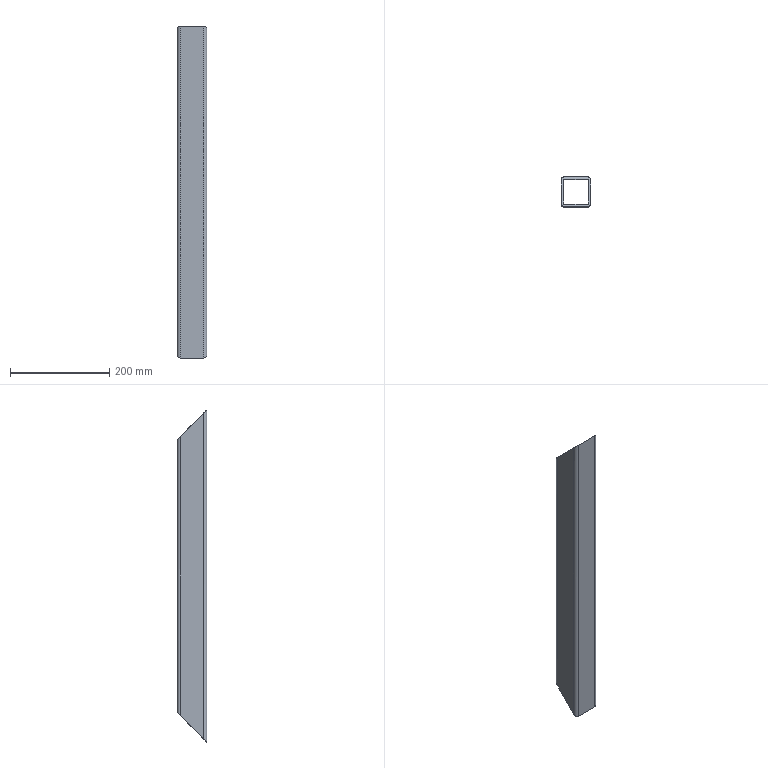Part | STEP file | Positioning_id1438_x_t | 1 solid | 14 faces | box 60 x 60 x 670 mm | volume 652149 mm3 | plane 10 | cylinder 4 | commonest cylinder face diameters 12 x4
STEP:
#1=CARTESIAN_POINT('',(0.,0.,0.));
#2=DIRECTION('',(0.,0.,1.));
#3=DIRECTION('',(1.,0.,0.));
#4=AXIS2_PLACEMENT_3D('',#1,#2,#3);
#5=CARTESIAN_POINT('',(-1086.002,-745.,-132.534));
#6=VERTEX_POINT('',#5);
#7=CARTESIAN_POINT('',(-1086.002,-695.,-82.534));
#8=VERTEX_POINT('',#7);
#9=CARTESIAN_POINT('',(-1086.002,-745.,-132.534));
#10=DIRECTION('',(0.,0.7071,0.7071));
#11=VECTOR('',#10,1.);
#12=LINE('',#9,#11);
#13=CARTESIAN_POINT('',(-1021.002,-750.,-137.534));
#14=DIRECTION('',(0.,-0.7071,0.7071));
#15=DIRECTION('',(0.,0.7071,0.7071));
#16=AXIS2_PLACEMENT_3D('',#13,#14,#15);
#17=PLANE('',#16);
#18=CARTESIAN_POINT('',(7.071,65.));
#19=DIRECTION('',(1.,0.));
#20=VECTOR('',#19,1.);
#21=LINE('',#18,#20);
#22=(GEOMETRIC_REPRESENTATION_CONTEXT(2)PARAMETRIC_REPRESENTATION_CONTEXT()REPRESENTATION_CONTEXT('',''));
#23=DEFINITIONAL_REPRESENTATION('',(#21),#22);
#24=PCURVE('',#17,#23);
#25=CARTESIAN_POINT('',(-1086.002,-745.,257.466));
#26=DIRECTION('',(-1.,0.,0.));
#27=DIRECTION('',(0.,1.,0.));
#28=AXIS2_PLACEMENT_3D('',#25,#26,#27);
#29=PLANE('',#28);
#30=CARTESIAN_POINT('',(0.,390.));
#31=DIRECTION('',(0.7071,-0.7071));
#32=VECTOR('',#31,1.);
#33=LINE('',#30,#32);
#34=(GEOMETRIC_REPRESENTATION_CONTEXT(2)PARAMETRIC_REPRESENTATION_CONTEXT()REPRESENTATION_CONTEXT('',''));
#35=DEFINITIONAL_REPRESENTATION('',(#33),#34);
#36=PCURVE('',#29,#35);
#37=SURFACE_CURVE('',#12,(#24,#36),.PCURVE_S1.);
#38=EDGE_CURVE('',#6,#8,#37,.T.);
#39=ORIENTED_EDGE('',*,*,#38,.F.);
#40=CARTESIAN_POINT('',(-1036.002,-745.,-132.534));
#41=VERTEX_POINT('',#40);
#42=CARTESIAN_POINT('',(-1036.002,-745.,-132.534));
#43=DIRECTION('',(-1.,0.,0.));
#44=VECTOR('',#43,1.);
#45=LINE('',#42,#44);
#46=CARTESIAN_POINT('',(7.071,15.));
#47=DIRECTION('',(0.,1.));
#48=VECTOR('',#47,1.);
#49=LINE('',#46,#48);
#50=(GEOMETRIC_REPRESENTATION_CONTEXT(2)PARAMETRIC_REPRESENTATION_CONTEXT()REPRESENTATION_CONTEXT('',''));
#51=DEFINITIONAL_REPRESENTATION('',(#49),#50);
#52=PCURVE('',#17,#51);
#53=CARTESIAN_POINT('',(-1061.002,-745.,257.466));
#54=DIRECTION('',(0.,-1.,0.));
#55=DIRECTION('',(-1.,0.,0.));
#56=AXIS2_PLACEMENT_3D('',#53,#54,#55);
#57=PLANE('',#56);
#58=CARTESIAN_POINT('',(-25.,390.));
#59=DIRECTION('',(1.,0.));
#60=VECTOR('',#59,1.);
#61=LINE('',#58,#60);
#62=(GEOMETRIC_REPRESENTATION_CONTEXT(2)PARAMETRIC_REPRESENTATION_CONTEXT()REPRESENTATION_CONTEXT('',''));
#63=DEFINITIONAL_REPRESENTATION('',(#61),#62);
#64=PCURVE('',#57,#63);
#65=SURFACE_CURVE('',#45,(#52,#64),.PCURVE_S1.);
#66=EDGE_CURVE('',#41,#6,#65,.T.);
#67=ORIENTED_EDGE('',*,*,#66,.F.);
#68=CARTESIAN_POINT('',(-1036.002,-695.,-82.534));
#69=VERTEX_POINT('',#68);
#70=CARTESIAN_POINT('',(-1036.002,-695.,-82.534));
#71=DIRECTION('',(0.,-0.7071,-0.7071));
#72=VECTOR('',#71,1.);
#73=LINE('',#70,#72);
#74=CARTESIAN_POINT('',(77.782,15.));
#75=DIRECTION('',(-1.,0.));
#76=VECTOR('',#75,1.);
#77=LINE('',#74,#76);
#78=(GEOMETRIC_REPRESENTATION_CONTEXT(2)PARAMETRIC_REPRESENTATION_CONTEXT()REPRESENTATION_CONTEXT('',''));
#79=DEFINITIONAL_REPRESENTATION('',(#77),#78);
#80=PCURVE('',#17,#79);
#81=CARTESIAN_POINT('',(-1036.002,-745.,257.466));
#82=DIRECTION('',(1.,0.,0.));
#83=DIRECTION('',(0.,-1.,0.));
#84=AXIS2_PLACEMENT_3D('',#81,#82,#83);
#85=PLANE('',#84);
#86=CARTESIAN_POINT('',(-50.,340.));
#87=DIRECTION('',(0.7071,0.7071));
#88=VECTOR('',#87,1.);
#89=LINE('',#86,#88);
#90=(GEOMETRIC_REPRESENTATION_CONTEXT(2)PARAMETRIC_REPRESENTATION_CONTEXT()REPRESENTATION_CONTEXT('',''));
#91=DEFINITIONAL_REPRESENTATION('',(#89),#90);
#92=PCURVE('',#85,#91);
#93=SURFACE_CURVE('',#73,(#80,#92),.PCURVE_S1.);
#94=EDGE_CURVE('',#69,#41,#93,.T.);
#95=ORIENTED_EDGE('',*,*,#94,.F.);
#96=CARTESIAN_POINT('',(-1086.002,-695.,-82.534));
#97=DIRECTION('',(1.,0.,0.));
#98=VECTOR('',#97,1.);
#99=LINE('',#96,#98);
#100=CARTESIAN_POINT('',(77.782,65.));
#101=DIRECTION('',(0.,-1.));
#102=VECTOR('',#101,1.);
#103=LINE('',#100,#102);
#104=(GEOMETRIC_REPRESENTATION_CONTEXT(2)PARAMETRIC_REPRESENTATION_CONTEXT()REPRESENTATION_CONTEXT('',''));
#105=DEFINITIONAL_REPRESENTATION('',(#103),#104);
#106=PCURVE('',#17,#105);
#107=CARTESIAN_POINT('',(-1061.002,-695.,257.466));
#108=DIRECTION('',(0.,1.,0.));
#109=DIRECTION('',(1.,0.,0.));
#110=AXIS2_PLACEMENT_3D('',#107,#108,#109);
#111=PLANE('',#110);
#112=CARTESIAN_POINT('',(-25.,340.));
#113=DIRECTION('',(1.,0.));
#114=VECTOR('',#113,1.);
#115=LINE('',#112,#114);
#116=(GEOMETRIC_REPRESENTATION_CONTEXT(2)PARAMETRIC_REPRESENTATION_CONTEXT()REPRESENTATION_CONTEXT('',''));
#117=DEFINITIONAL_REPRESENTATION('',(#115),#116);
#118=PCURVE('',#111,#117);
#119=SURFACE_CURVE('',#99,(#106,#118),.PCURVE_S1.);
#120=EDGE_CURVE('',#8,#69,#119,.T.);
#121=ORIENTED_EDGE('',*,*,#120,.F.);
#122=EDGE_LOOP('',(#39,#67,#95,#121));
#123=FACE_BOUND('',#122,.T.);
#124=CARTESIAN_POINT('',(-1085.002,-690.,-77.534));
#125=VERTEX_POINT('',#124);
#126=CARTESIAN_POINT('',(-1037.002,-690.,-77.534));
#127=VERTEX_POINT('',#126);
#128=CARTESIAN_POINT('',(-1085.002,-690.,-77.534));
#129=DIRECTION('',(1.,0.,0.));
#130=VECTOR('',#129,1.);
#131=LINE('',#128,#130);
#132=CARTESIAN_POINT('',(84.853,64.));
#133=DIRECTION('',(0.,-1.));
#134=VECTOR('',#133,1.);
#135=LINE('',#132,#134);
#136=(GEOMETRIC_REPRESENTATION_CONTEXT(2)PARAMETRIC_REPRESENTATION_CONTEXT()REPRESENTATION_CONTEXT('',''));
#137=DEFINITIONAL_REPRESENTATION('',(#135),#136);
#138=PCURVE('',#17,#137);
#139=CARTESIAN_POINT('',(-1061.002,-690.,257.466));
#140=DIRECTION('',(0.,1.,0.));
#141=DIRECTION('',(1.,0.,0.));
#142=AXIS2_PLACEMENT_3D('',#139,#140,#141);
#143=PLANE('',#142);
#144=CARTESIAN_POINT('',(-24.,335.));
#145=DIRECTION('',(1.,0.));
#146=VECTOR('',#145,1.);
#147=LINE('',#144,#146);
#148=(GEOMETRIC_REPRESENTATION_CONTEXT(2)PARAMETRIC_REPRESENTATION_CONTEXT()REPRESENTATION_CONTEXT('',''));
#149=DEFINITIONAL_REPRESENTATION('',(#147),#148);
#150=PCURVE('',#143,#149);
#151=SURFACE_CURVE('',#131,(#138,#150),.PCURVE_S1.);
#152=EDGE_CURVE('',#125,#127,#151,.T.);
#153=ORIENTED_EDGE('',*,*,#152,.T.);
#154=CARTESIAN_POINT('',(-1031.002,-696.,-83.534));
#155=VERTEX_POINT('',#154);
#156=CARTESIAN_POINT('',(-1037.002,-696.,-83.534));
#157=DIRECTION('',(0.,0.7071,-0.7071));
#158=DIRECTION('',(0.,-0.7071,-0.7071));
#159=AXIS2_PLACEMENT_3D('',#156,#157,#158);
#160=ELLIPSE('',#159,8.485,6.);
#161=CARTESIAN_POINT('',(67.882,16.));
#162=CARTESIAN_POINT('',(67.882,26.392));
#163=CARTESIAN_POINT('',(80.61,21.196));
#164=CARTESIAN_POINT('',(93.338,16.));
#165=CARTESIAN_POINT('',(80.61,10.804));
#166=CARTESIAN_POINT('',(67.882,5.608));
#167=CARTESIAN_POINT('',(67.882,16.));
#168=(BOUNDED_CURVE()B_SPLINE_CURVE(2,(#161,#162,#163,#164,#165,#166,#167),.UNSPECIFIED.,.T.,.F.)B_SPLINE_CURVE_WITH_KNOTS((1,2,2,2,2,1),(-2.094,0.,2.094,4.189,6.283,8.378),.UNSPECIFIED.)CURVE()GEOMETRIC_REPRESENTATION_ITEM()RATIONAL_B_SPLINE_CURVE((1.,0.5,1.,0.5,1.,0.5,1.))REPRESENTATION_ITEM(''));
#169=(GEOMETRIC_REPRESENTATION_CONTEXT(2)PARAMETRIC_REPRESENTATION_CONTEXT()REPRESENTATION_CONTEXT('',''));
#170=DEFINITIONAL_REPRESENTATION('',(#168),#169);
#171=PCURVE('',#17,#170);
#172=CARTESIAN_POINT('',(-1037.002,-696.,257.466));
#173=DIRECTION('',(0.,0.,-1.));
#174=DIRECTION('',(-1.,0.,0.));
#175=AXIS2_PLACEMENT_3D('',#172,#173,#174);
#176=CYLINDRICAL_SURFACE('',#175,6.);
#177=CARTESIAN_POINT('',(1.571,335.));
#178=CARTESIAN_POINT('',(1.595,335.));
#179=CARTESIAN_POINT('',(1.642,335.01));
#180=CARTESIAN_POINT('',(1.714,335.056));
#181=CARTESIAN_POINT('',(1.785,335.132));
#182=CARTESIAN_POINT('',(1.856,335.238));
#183=CARTESIAN_POINT('',(1.928,335.374));
#184=CARTESIAN_POINT('',(1.999,335.538));
#185=CARTESIAN_POINT('',(2.071,335.729));
#186=CARTESIAN_POINT('',(2.142,335.948));
#187=CARTESIAN_POINT('',(2.213,336.193));
#188=CARTESIAN_POINT('',(2.285,336.462));
#189=CARTESIAN_POINT('',(2.356,336.754));
#190=CARTESIAN_POINT('',(2.428,337.067));
#191=CARTESIAN_POINT('',(2.499,337.401));
#192=CARTESIAN_POINT('',(2.57,337.753));
#193=CARTESIAN_POINT('',(2.642,338.122));
#194=CARTESIAN_POINT('',(2.713,338.505));
#195=CARTESIAN_POINT('',(2.785,338.901));
#196=CARTESIAN_POINT('',(2.856,339.308));
#197=CARTESIAN_POINT('',(2.927,339.724));
#198=CARTESIAN_POINT('',(2.999,340.145));
#199=CARTESIAN_POINT('',(3.07,340.572));
#200=CARTESIAN_POINT('',(3.118,340.857));
#201=CARTESIAN_POINT('',(3.142,341.));
#202=B_SPLINE_CURVE_WITH_KNOTS('',3,(#177,#178,#179,#180,#181,#182,#183,#184,#185,#186,#187,#188,#189,#190,#191,#192,#193,#194,#195,#196,#197,#198,#199,#200,#201),.UNSPECIFIED.,.F.,.F.,(4,1,1,1,1,1,1,1,1,1,1,1,1,1,1,1,1,1,1,1,1,1,4),(3.142,3.213,3.284,3.356,3.427,3.499,3.57,3.641,3.713,3.784,3.856,3.927,3.998,4.07,4.141,4.213,4.284,4.355,4.427,4.498,4.57,4.641,4.712),.QUASI_UNIFORM_KNOTS.);
#203=(GEOMETRIC_REPRESENTATION_CONTEXT(2)PARAMETRIC_REPRESENTATION_CONTEXT()REPRESENTATION_CONTEXT('',''));
#204=DEFINITIONAL_REPRESENTATION('',(#202),#203);
#205=PCURVE('',#176,#204);
#206=SURFACE_CURVE('',#160,(#171,#205),.PCURVE_S1.);
#207=EDGE_CURVE('',#127,#155,#206,.T.);
#208=ORIENTED_EDGE('',*,*,#207,.T.);
#209=CARTESIAN_POINT('',(-1031.002,-744.,-131.534));
#210=VERTEX_POINT('',#209);
#211=CARTESIAN_POINT('',(-1031.002,-696.,-83.534));
#212=DIRECTION('',(0.,-0.7071,-0.7071));
#213=VECTOR('',#212,1.);
#214=LINE('',#211,#213);
#215=CARTESIAN_POINT('',(76.368,10.));
#216=DIRECTION('',(-1.,0.));
#217=VECTOR('',#216,1.);
#218=LINE('',#215,#217);
#219=(GEOMETRIC_REPRESENTATION_CONTEXT(2)PARAMETRIC_REPRESENTATION_CONTEXT()REPRESENTATION_CONTEXT('',''));
#220=DEFINITIONAL_REPRESENTATION('',(#218),#219);
#221=PCURVE('',#17,#220);
#222=CARTESIAN_POINT('',(-1031.002,-750.,257.466));
#223=DIRECTION('',(1.,0.,0.));
#224=DIRECTION('',(0.,-1.,0.));
#225=AXIS2_PLACEMENT_3D('',#222,#223,#224);
#226=PLANE('',#225);
#227=CARTESIAN_POINT('',(-54.,341.));
#228=DIRECTION('',(0.7071,0.7071));
#229=VECTOR('',#228,1.);
#230=LINE('',#227,#229);
#231=(GEOMETRIC_REPRESENTATION_CONTEXT(2)PARAMETRIC_REPRESENTATION_CONTEXT()REPRESENTATION_CONTEXT('',''));
#232=DEFINITIONAL_REPRESENTATION('',(#230),#231);
#233=PCURVE('',#226,#232);
#234=SURFACE_CURVE('',#214,(#221,#233),.PCURVE_S1.);
#235=EDGE_CURVE('',#155,#210,#234,.T.);
#236=ORIENTED_EDGE('',*,*,#235,.T.);
#237=CARTESIAN_POINT('',(-1037.002,-750.,-137.534));
#238=VERTEX_POINT('',#237);
#239=CARTESIAN_POINT('',(-1037.002,-744.,-131.534));
#240=DIRECTION('',(0.,0.7071,-0.7071));
#241=DIRECTION('',(0.,0.7071,0.7071));
#242=AXIS2_PLACEMENT_3D('',#239,#240,#241);
#243=ELLIPSE('',#242,8.485,6.);
#244=CARTESIAN_POINT('',(16.971,16.));
#245=CARTESIAN_POINT('',(16.971,5.608));
#246=CARTESIAN_POINT('',(4.243,10.804));
#247=CARTESIAN_POINT('',(-8.485,16.));
#248=CARTESIAN_POINT('',(4.243,21.196));
#249=CARTESIAN_POINT('',(16.971,26.392));
#250=CARTESIAN_POINT('',(16.971,16.));
#251=(BOUNDED_CURVE()B_SPLINE_CURVE(2,(#244,#245,#246,#247,#248,#249,#250),.UNSPECIFIED.,.T.,.F.)B_SPLINE_CURVE_WITH_KNOTS((1,2,2,2,2,1),(-2.094,0.,2.094,4.189,6.283,8.378),.UNSPECIFIED.)CURVE()GEOMETRIC_REPRESENTATION_ITEM()RATIONAL_B_SPLINE_CURVE((1.,0.5,1.,0.5,1.,0.5,1.))REPRESENTATION_ITEM(''));
#252=(GEOMETRIC_REPRESENTATION_CONTEXT(2)PARAMETRIC_REPRESENTATION_CONTEXT()REPRESENTATION_CONTEXT('',''));
#253=DEFINITIONAL_REPRESENTATION('',(#251),#252);
#254=PCURVE('',#17,#253);
#255=CARTESIAN_POINT('',(-1037.002,-744.,257.466));
#256=DIRECTION('',(0.,0.,1.));
#257=DIRECTION('',(1.,0.,0.));
#258=AXIS2_PLACEMENT_3D('',#255,#256,#257);
#259=CYLINDRICAL_SURFACE('',#258,6.);
#260=CARTESIAN_POINT('',(6.283,-389.));
#261=CARTESIAN_POINT('',(6.259,-389.143));
#262=CARTESIAN_POINT('',(6.212,-389.428));
#263=CARTESIAN_POINT('',(6.14,-389.855));
#264=CARTESIAN_POINT('',(6.069,-390.276));
#265=CARTESIAN_POINT('',(5.998,-390.692));
#266=CARTESIAN_POINT('',(5.926,-391.099));
#267=CARTESIAN_POINT('',(5.855,-391.495));
#268=CARTESIAN_POINT('',(5.783,-391.878));
#269=CARTESIAN_POINT('',(5.712,-392.247));
#270=CARTESIAN_POINT('',(5.641,-392.599));
#271=CARTESIAN_POINT('',(5.569,-392.933));
#272=CARTESIAN_POINT('',(5.498,-393.246));
#273=CARTESIAN_POINT('',(5.426,-393.538));
#274=CARTESIAN_POINT('',(5.355,-393.807));
#275=CARTESIAN_POINT('',(5.284,-394.052));
#276=CARTESIAN_POINT('',(5.212,-394.271));
#277=CARTESIAN_POINT('',(5.141,-394.462));
#278=CARTESIAN_POINT('',(5.069,-394.626));
#279=CARTESIAN_POINT('',(4.998,-394.762));
#280=CARTESIAN_POINT('',(4.927,-394.868));
#281=CARTESIAN_POINT('',(4.855,-394.944));
#282=CARTESIAN_POINT('',(4.784,-394.99));
#283=CARTESIAN_POINT('',(4.736,-395.));
#284=CARTESIAN_POINT('',(4.712,-395.));
#285=B_SPLINE_CURVE_WITH_KNOTS('',3,(#260,#261,#262,#263,#264,#265,#266,#267,#268,#269,#270,#271,#272,#273,#274,#275,#276,#277,#278,#279,#280,#281,#282,#283,#284),.UNSPECIFIED.,.F.,.F.,(4,1,1,1,1,1,1,1,1,1,1,1,1,1,1,1,1,1,1,1,1,1,4),(1.571,1.642,1.714,1.785,1.856,1.928,1.999,2.071,2.142,2.213,2.285,2.356,2.428,2.499,2.57,2.642,2.713,2.785,2.856,2.927,2.999,3.07,3.142),.QUASI_UNIFORM_KNOTS.);
#286=(GEOMETRIC_REPRESENTATION_CONTEXT(2)PARAMETRIC_REPRESENTATION_CONTEXT()REPRESENTATION_CONTEXT('',''));
#287=DEFINITIONAL_REPRESENTATION('',(#285),#286);
#288=PCURVE('',#259,#287);
#289=SURFACE_CURVE('',#243,(#254,#288),.PCURVE_S1.);
#290=EDGE_CURVE('',#210,#238,#289,.T.);
#291=ORIENTED_EDGE('',*,*,#290,.T.);
#292=CARTESIAN_POINT('',(-1085.002,-750.,-137.534));
#293=VERTEX_POINT('',#292);
#294=CARTESIAN_POINT('',(-1037.002,-750.,-137.534));
#295=DIRECTION('',(-1.,0.,0.));
#296=VECTOR('',#295,1.);
#297=LINE('',#294,#296);
#298=CARTESIAN_POINT('',(0.,16.));
#299=DIRECTION('',(0.,1.));
#300=VECTOR('',#299,1.);
#301=LINE('',#298,#300);
#302=(GEOMETRIC_REPRESENTATION_CONTEXT(2)PARAMETRIC_REPRESENTATION_CONTEXT()REPRESENTATION_CONTEXT('',''));
#303=DEFINITIONAL_REPRESENTATION('',(#301),#302);
#304=PCURVE('',#17,#303);
#305=CARTESIAN_POINT('',(-1061.002,-750.,257.466));
#306=DIRECTION('',(0.,-1.,0.));
#307=DIRECTION('',(-1.,0.,0.));
#308=AXIS2_PLACEMENT_3D('',#305,#306,#307);
#309=PLANE('',#308);
#310=CARTESIAN_POINT('',(-24.,395.));
#311=DIRECTION('',(1.,0.));
#312=VECTOR('',#311,1.);
#313=LINE('',#310,#312);
#314=(GEOMETRIC_REPRESENTATION_CONTEXT(2)PARAMETRIC_REPRESENTATION_CONTEXT()REPRESENTATION_CONTEXT('',''));
#315=DEFINITIONAL_REPRESENTATION('',(#313),#314);
#316=PCURVE('',#309,#315);
#317=SURFACE_CURVE('',#297,(#304,#316),.PCURVE_S1.);
#318=EDGE_CURVE('',#238,#293,#317,.T.);
#319=ORIENTED_EDGE('',*,*,#318,.T.);
#320=CARTESIAN_POINT('',(-1091.002,-744.,-131.534));
#321=VERTEX_POINT('',#320);
#322=CARTESIAN_POINT('',(-1085.002,-744.,-131.534));
#323=DIRECTION('',(0.,0.7071,-0.7071));
#324=DIRECTION('',(0.,-0.7071,-0.7071));
#325=AXIS2_PLACEMENT_3D('',#322,#323,#324);
#326=ELLIPSE('',#325,8.485,6.);
#327=CARTESIAN_POINT('',(0.,64.));
#328=CARTESIAN_POINT('',(0.,74.392));
#329=CARTESIAN_POINT('',(12.728,69.196));
#330=CARTESIAN_POINT('',(25.456,64.));
#331=CARTESIAN_POINT('',(12.728,58.804));
#332=CARTESIAN_POINT('',(0.,53.608));
#333=CARTESIAN_POINT('',(0.,64.));
#334=(BOUNDED_CURVE()B_SPLINE_CURVE(2,(#327,#328,#329,#330,#331,#332,#333),.UNSPECIFIED.,.T.,.F.)B_SPLINE_CURVE_WITH_KNOTS((1,2,2,2,2,1),(-2.094,0.,2.094,4.189,6.283,8.378),.UNSPECIFIED.)CURVE()GEOMETRIC_REPRESENTATION_ITEM()RATIONAL_B_SPLINE_CURVE((1.,0.5,1.,0.5,1.,0.5,1.))REPRESENTATION_ITEM(''));
#335=(GEOMETRIC_REPRESENTATION_CONTEXT(2)PARAMETRIC_REPRESENTATION_CONTEXT()REPRESENTATION_CONTEXT('',''));
#336=DEFINITIONAL_REPRESENTATION('',(#334),#335);
#337=PCURVE('',#17,#336);
#338=CARTESIAN_POINT('',(-1085.002,-744.,257.466));
#339=DIRECTION('',(0.,0.,-1.));
#340=DIRECTION('',(-1.,0.,0.));
#341=AXIS2_PLACEMENT_3D('',#338,#339,#340);
#342=CYLINDRICAL_SURFACE('',#341,6.);
#343=CARTESIAN_POINT('',(4.712,395.));
#344=CARTESIAN_POINT('',(4.736,395.));
#345=CARTESIAN_POINT('',(4.784,394.99));
#346=CARTESIAN_POINT('',(4.855,394.944));
#347=CARTESIAN_POINT('',(4.927,394.868));
#348=CARTESIAN_POINT('',(4.998,394.762));
#349=CARTESIAN_POINT('',(5.069,394.626));
#350=CARTESIAN_POINT('',(5.141,394.462));
#351=CARTESIAN_POINT('',(5.212,394.271));
#352=CARTESIAN_POINT('',(5.284,394.052));
#353=CARTESIAN_POINT('',(5.355,393.807));
#354=CARTESIAN_POINT('',(5.426,393.538));
#355=CARTESIAN_POINT('',(5.498,393.246));
#356=CARTESIAN_POINT('',(5.569,392.933));
#357=CARTESIAN_POINT('',(5.641,392.599));
#358=CARTESIAN_POINT('',(5.712,392.247));
#359=CARTESIAN_POINT('',(5.783,391.878));
#360=CARTESIAN_POINT('',(5.855,391.495));
#361=CARTESIAN_POINT('',(5.926,391.099));
#362=CARTESIAN_POINT('',(5.998,390.692));
#363=CARTESIAN_POINT('',(6.069,390.276));
#364=CARTESIAN_POINT('',(6.14,389.855));
#365=CARTESIAN_POINT('',(6.212,389.428));
#366=CARTESIAN_POINT('',(6.259,389.143));
#367=CARTESIAN_POINT('',(6.283,389.));
#368=B_SPLINE_CURVE_WITH_KNOTS('',3,(#343,#344,#345,#346,#347,#348,#349,#350,#351,#352,#353,#354,#355,#356,#357,#358,#359,#360,#361,#362,#363,#364,#365,#366,#367),.UNSPECIFIED.,.F.,.F.,(4,1,1,1,1,1,1,1,1,1,1,1,1,1,1,1,1,1,1,1,1,1,4),(0.,0.0714,0.1428,0.2142,0.2856,0.357,0.4284,0.4998,0.5712,0.6426,0.714,0.7854,0.8568,0.9282,0.9996,1.071,1.142,1.214,1.285,1.357,1.428,1.499,1.571),.QUASI_UNIFORM_KNOTS.);
#369=(GEOMETRIC_REPRESENTATION_CONTEXT(2)PARAMETRIC_REPRESENTATION_CONTEXT()REPRESENTATION_CONTEXT('',''));
#370=DEFINITIONAL_REPRESENTATION('',(#368),#369);
#371=PCURVE('',#342,#370);
#372=SURFACE_CURVE('',#326,(#337,#371),.PCURVE_S1.);
#373=EDGE_CURVE('',#293,#321,#372,.T.);
#374=ORIENTED_EDGE('',*,*,#373,.T.);
#375=CARTESIAN_POINT('',(-1091.002,-696.,-83.534));
#376=VERTEX_POINT('',#375);
#377=CARTESIAN_POINT('',(-1091.002,-744.,-131.534));
#378=DIRECTION('',(0.,0.7071,0.7071));
#379=VECTOR('',#378,1.);
#380=LINE('',#377,#379);
#381=CARTESIAN_POINT('',(8.485,70.));
#382=DIRECTION('',(1.,0.));
#383=VECTOR('',#382,1.);
#384=LINE('',#381,#383);
#385=(GEOMETRIC_REPRESENTATION_CONTEXT(2)PARAMETRIC_REPRESENTATION_CONTEXT()REPRESENTATION_CONTEXT('',''));
#386=DEFINITIONAL_REPRESENTATION('',(#384),#385);
#387=PCURVE('',#17,#386);
#388=CARTESIAN_POINT('',(-1091.002,-750.,257.466));
#389=DIRECTION('',(-1.,0.,0.));
#390=DIRECTION('',(0.,1.,0.));
#391=AXIS2_PLACEMENT_3D('',#388,#389,#390);
#392=PLANE('',#391);
#393=CARTESIAN_POINT('',(6.,389.));
#394=DIRECTION('',(0.7071,-0.7071));
#395=VECTOR('',#394,1.);
#396=LINE('',#393,#395);
#397=(GEOMETRIC_REPRESENTATION_CONTEXT(2)PARAMETRIC_REPRESENTATION_CONTEXT()REPRESENTATION_CONTEXT('',''));
#398=DEFINITIONAL_REPRESENTATION('',(#396),#397);
#399=PCURVE('',#392,#398);
#400=SURFACE_CURVE('',#380,(#387,#399),.PCURVE_S1.);
#401=EDGE_CURVE('',#321,#376,#400,.T.);
#402=ORIENTED_EDGE('',*,*,#401,.T.);
#403=CARTESIAN_POINT('',(-1085.002,-696.,-83.534));
#404=DIRECTION('',(0.,0.7071,-0.7071));
#405=DIRECTION('',(0.,0.7071,0.7071));
#406=AXIS2_PLACEMENT_3D('',#403,#404,#405);
#407=ELLIPSE('',#406,8.485,6.);
#408=CARTESIAN_POINT('',(84.853,64.));
#409=CARTESIAN_POINT('',(84.853,53.608));
#410=CARTESIAN_POINT('',(72.125,58.804));
#411=CARTESIAN_POINT('',(59.397,64.));
#412=CARTESIAN_POINT('',(72.125,69.196));
#413=CARTESIAN_POINT('',(84.853,74.392));
#414=CARTESIAN_POINT('',(84.853,64.));
#415=(BOUNDED_CURVE()B_SPLINE_CURVE(2,(#408,#409,#410,#411,#412,#413,#414),.UNSPECIFIED.,.T.,.F.)B_SPLINE_CURVE_WITH_KNOTS((1,2,2,2,2,1),(-2.094,0.,2.094,4.189,6.283,8.378),.UNSPECIFIED.)CURVE()GEOMETRIC_REPRESENTATION_ITEM()RATIONAL_B_SPLINE_CURVE((1.,0.5,1.,0.5,1.,0.5,1.))REPRESENTATION_ITEM(''));
#416=(GEOMETRIC_REPRESENTATION_CONTEXT(2)PARAMETRIC_REPRESENTATION_CONTEXT()REPRESENTATION_CONTEXT('',''));
#417=DEFINITIONAL_REPRESENTATION('',(#415),#416);
#418=PCURVE('',#17,#417);
#419=CARTESIAN_POINT('',(-1085.002,-696.,257.466));
#420=DIRECTION('',(0.,0.,1.));
#421=DIRECTION('',(1.,0.,0.));
#422=AXIS2_PLACEMENT_3D('',#419,#420,#421);
#423=CYLINDRICAL_SURFACE('',#422,6.);
#424=CARTESIAN_POINT('',(3.142,-341.));
#425=CARTESIAN_POINT('',(3.118,-340.857));
#426=CARTESIAN_POINT('',(3.07,-340.572));
#427=CARTESIAN_POINT('',(2.999,-340.145));
#428=CARTESIAN_POINT('',(2.927,-339.724));
#429=CARTESIAN_POINT('',(2.856,-339.308));
#430=CARTESIAN_POINT('',(2.785,-338.901));
#431=CARTESIAN_POINT('',(2.713,-338.505));
#432=CARTESIAN_POINT('',(2.642,-338.122));
#433=CARTESIAN_POINT('',(2.57,-337.753));
#434=CARTESIAN_POINT('',(2.499,-337.401));
#435=CARTESIAN_POINT('',(2.428,-337.067));
#436=CARTESIAN_POINT('',(2.356,-336.754));
#437=CARTESIAN_POINT('',(2.285,-336.462));
#438=CARTESIAN_POINT('',(2.213,-336.193));
#439=CARTESIAN_POINT('',(2.142,-335.948));
#440=CARTESIAN_POINT('',(2.071,-335.729));
#441=CARTESIAN_POINT('',(1.999,-335.538));
#442=CARTESIAN_POINT('',(1.928,-335.374));
#443=CARTESIAN_POINT('',(1.856,-335.238));
#444=CARTESIAN_POINT('',(1.785,-335.132));
#445=CARTESIAN_POINT('',(1.714,-335.056));
#446=CARTESIAN_POINT('',(1.642,-335.01));
#447=CARTESIAN_POINT('',(1.595,-335.));
#448=CARTESIAN_POINT('',(1.571,-335.));
#449=B_SPLINE_CURVE_WITH_KNOTS('',3,(#424,#425,#426,#427,#428,#429,#430,#431,#432,#433,#434,#435,#436,#437,#438,#439,#440,#441,#442,#443,#444,#445,#446,#447,#448),.UNSPECIFIED.,.F.,.F.,(4,1,1,1,1,1,1,1,1,1,1,1,1,1,1,1,1,1,1,1,1,1,4),(4.712,4.784,4.855,4.927,4.998,5.069,5.141,5.212,5.284,5.355,5.426,5.498,5.569,5.641,5.712,5.783,5.855,5.926,5.998,6.069,6.14,6.212,6.283),.QUASI_UNIFORM_KNOTS.);
#450=(GEOMETRIC_REPRESENTATION_CONTEXT(2)PARAMETRIC_REPRESENTATION_CONTEXT()REPRESENTATION_CONTEXT('',''));
#451=DEFINITIONAL_REPRESENTATION('',(#449),#450);
#452=PCURVE('',#423,#451);
#453=SURFACE_CURVE('',#407,(#418,#452),.PCURVE_S1.);
#454=EDGE_CURVE('',#376,#125,#453,.T.);
#455=ORIENTED_EDGE('',*,*,#454,.T.);
#456=EDGE_LOOP('',(#153,#208,#236,#291,#319,#374,#402,#455));
#457=FACE_BOUND('',#456,.T.);
#458=ADVANCED_FACE('',(#123,#457),#17,.F.);
#459=CARTESIAN_POINT('',(-1091.002,-744.,526.466));
#460=VERTEX_POINT('',#459);
#461=CARTESIAN_POINT('',(-1091.002,-744.,-131.534));
#462=DIRECTION('',(0.,0.,1.));
#463=VECTOR('',#462,1.);
#464=LINE('',#461,#463);
#465=CARTESIAN_POINT('',(6.283,389.));
#466=DIRECTION('',(0.,-1.));
#467=VECTOR('',#466,1.);
#468=LINE('',#465,#467);
#469=(GEOMETRIC_REPRESENTATION_CONTEXT(2)PARAMETRIC_REPRESENTATION_CONTEXT()REPRESENTATION_CONTEXT('',''));
#470=DEFINITIONAL_REPRESENTATION('',(#468),#469);
#471=PCURVE('',#342,#470);
#472=CARTESIAN_POINT('',(6.,389.));
#473=DIRECTION('',(0.,-1.));
#474=VECTOR('',#473,1.);
#475=LINE('',#472,#474);
#476=(GEOMETRIC_REPRESENTATION_CONTEXT(2)PARAMETRIC_REPRESENTATION_CONTEXT()REPRESENTATION_CONTEXT('',''));
#477=DEFINITIONAL_REPRESENTATION('',(#475),#476);
#478=PCURVE('',#392,#477);
#479=SURFACE_CURVE('',#464,(#471,#478),.PCURVE_S1.);
#480=EDGE_CURVE('',#321,#460,#479,.T.);
#481=ORIENTED_EDGE('',*,*,#480,.F.);
#482=ORIENTED_EDGE('',*,*,#373,.F.);
#483=CARTESIAN_POINT('',(-1085.002,-750.,532.466));
#484=VERTEX_POINT('',#483);
#485=CARTESIAN_POINT('',(-1085.002,-750.,532.466));
#486=DIRECTION('',(0.,0.,-1.));
#487=VECTOR('',#486,1.);
#488=LINE('',#485,#487);
#489=CARTESIAN_POINT('',(4.712,-275.));
#490=DIRECTION('',(0.,1.));
#491=VECTOR('',#490,1.);
#492=LINE('',#489,#491);
#493=(GEOMETRIC_REPRESENTATION_CONTEXT(2)PARAMETRIC_REPRESENTATION_CONTEXT()REPRESENTATION_CONTEXT('',''));
#494=DEFINITIONAL_REPRESENTATION('',(#492),#493);
#495=PCURVE('',#342,#494);
#496=CARTESIAN_POINT('',(24.,-275.));
#497=DIRECTION('',(0.,1.));
#498=VECTOR('',#497,1.);
#499=LINE('',#496,#498);
#500=(GEOMETRIC_REPRESENTATION_CONTEXT(2)PARAMETRIC_REPRESENTATION_CONTEXT()REPRESENTATION_CONTEXT('',''));
#501=DEFINITIONAL_REPRESENTATION('',(#499),#500);
#502=PCURVE('',#309,#501);
#503=SURFACE_CURVE('',#488,(#495,#502),.PCURVE_S1.);
#504=EDGE_CURVE('',#484,#293,#503,.T.);
#505=ORIENTED_EDGE('',*,*,#504,.F.);
#506=CARTESIAN_POINT('',(-1085.002,-744.,526.466));
#507=DIRECTION('',(0.,0.7071,0.7071));
#508=DIRECTION('',(0.,0.7071,-0.7071));
#509=AXIS2_PLACEMENT_3D('',#506,#507,#508);
#510=ELLIPSE('',#509,8.485,6.);
#511=CARTESIAN_POINT('',(6.283,-269.));
#512=CARTESIAN_POINT('',(6.259,-269.143));
#513=CARTESIAN_POINT('',(6.212,-269.428));
#514=CARTESIAN_POINT('',(6.14,-269.855));
#515=CARTESIAN_POINT('',(6.069,-270.276));
#516=CARTESIAN_POINT('',(5.998,-270.692));
#517=CARTESIAN_POINT('',(5.926,-271.099));
#518=CARTESIAN_POINT('',(5.855,-271.495));
#519=CARTESIAN_POINT('',(5.783,-271.878));
#520=CARTESIAN_POINT('',(5.712,-272.247));
#521=CARTESIAN_POINT('',(5.641,-272.599));
#522=CARTESIAN_POINT('',(5.569,-272.933));
#523=CARTESIAN_POINT('',(5.498,-273.246));
#524=CARTESIAN_POINT('',(5.426,-273.538));
#525=CARTESIAN_POINT('',(5.355,-273.807));
#526=CARTESIAN_POINT('',(5.284,-274.052));
#527=CARTESIAN_POINT('',(5.212,-274.271));
#528=CARTESIAN_POINT('',(5.141,-274.462));
#529=CARTESIAN_POINT('',(5.069,-274.626));
#530=CARTESIAN_POINT('',(4.998,-274.762));
#531=CARTESIAN_POINT('',(4.927,-274.868));
#532=CARTESIAN_POINT('',(4.855,-274.944));
#533=CARTESIAN_POINT('',(4.784,-274.99));
#534=CARTESIAN_POINT('',(4.736,-275.));
#535=CARTESIAN_POINT('',(4.712,-275.));
#536=B_SPLINE_CURVE_WITH_KNOTS('',3,(#511,#512,#513,#514,#515,#516,#517,#518,#519,#520,#521,#522,#523,#524,#525,#526,#527,#528,#529,#530,#531,#532,#533,#534,#535),.UNSPECIFIED.,.F.,.F.,(4,1,1,1,1,1,1,1,1,1,1,1,1,1,1,1,1,1,1,1,1,1,4),(1.571,1.642,1.714,1.785,1.856,1.928,1.999,2.071,2.142,2.213,2.285,2.356,2.428,2.499,2.57,2.642,2.713,2.785,2.856,2.927,2.999,3.07,3.142),.QUASI_UNIFORM_KNOTS.);
#537=(GEOMETRIC_REPRESENTATION_CONTEXT(2)PARAMETRIC_REPRESENTATION_CONTEXT()REPRESENTATION_CONTEXT('',''));
#538=DEFINITIONAL_REPRESENTATION('',(#536),#537);
#539=PCURVE('',#342,#538);
#540=CARTESIAN_POINT('',(-1031.002,-750.,532.466));
#541=DIRECTION('',(0.,0.7071,0.7071));
#542=DIRECTION('',(0.,0.7071,-0.7071));
#543=AXIS2_PLACEMENT_3D('',#540,#541,#542);
#544=PLANE('',#543);
#545=CARTESIAN_POINT('',(8.485,54.));
#546=DIRECTION('',(1.,0.));
#547=AXIS2_PLACEMENT_2D('',#545,#546);
#548=ELLIPSE('',#547,8.485,6.);
#549=(GEOMETRIC_REPRESENTATION_CONTEXT(2)PARAMETRIC_REPRESENTATION_CONTEXT()REPRESENTATION_CONTEXT('',''));
#550=DEFINITIONAL_REPRESENTATION('',(#548),#549);
#551=PCURVE('',#544,#550);
#552=SURFACE_CURVE('',#510,(#539,#551),.PCURVE_S1.);
#553=EDGE_CURVE('',#460,#484,#552,.T.);
#554=ORIENTED_EDGE('',*,*,#553,.F.);
#555=EDGE_LOOP('',(#481,#482,#505,#554));
#556=FACE_BOUND('',#555,.T.);
#557=ADVANCED_FACE('',(#556),#342,.T.);
#558=CARTESIAN_POINT('',(-1037.002,-750.,532.466));
#559=VERTEX_POINT('',#558);
#560=CARTESIAN_POINT('',(-1037.002,-750.,-137.534));
#561=DIRECTION('',(0.,0.,1.));
#562=VECTOR('',#561,1.);
#563=LINE('',#560,#562);
#564=CARTESIAN_POINT('',(4.712,-395.));
#565=DIRECTION('',(0.,1.));
#566=VECTOR('',#565,1.);
#567=LINE('',#564,#566);
#568=(GEOMETRIC_REPRESENTATION_CONTEXT(2)PARAMETRIC_REPRESENTATION_CONTEXT()REPRESENTATION_CONTEXT('',''));
#569=DEFINITIONAL_REPRESENTATION('',(#567),#568);
#570=PCURVE('',#259,#569);
#571=CARTESIAN_POINT('',(-24.,395.));
#572=DIRECTION('',(0.,-1.));
#573=VECTOR('',#572,1.);
#574=LINE('',#571,#573);
#575=(GEOMETRIC_REPRESENTATION_CONTEXT(2)PARAMETRIC_REPRESENTATION_CONTEXT()REPRESENTATION_CONTEXT('',''));
#576=DEFINITIONAL_REPRESENTATION('',(#574),#575);
#577=PCURVE('',#309,#576);
#578=SURFACE_CURVE('',#563,(#570,#577),.PCURVE_S1.);
#579=EDGE_CURVE('',#238,#559,#578,.T.);
#580=ORIENTED_EDGE('',*,*,#579,.F.);
#581=ORIENTED_EDGE('',*,*,#290,.F.);
#582=CARTESIAN_POINT('',(-1031.002,-744.,526.466));
#583=VERTEX_POINT('',#582);
#584=CARTESIAN_POINT('',(-1031.002,-744.,526.466));
#585=DIRECTION('',(0.,0.,-1.));
#586=VECTOR('',#585,1.);
#587=LINE('',#584,#586);
#588=CARTESIAN_POINT('',(6.283,269.));
#589=DIRECTION('',(0.,-1.));
#590=VECTOR('',#589,1.);
#591=LINE('',#588,#590);
#592=(GEOMETRIC_REPRESENTATION_CONTEXT(2)PARAMETRIC_REPRESENTATION_CONTEXT()REPRESENTATION_CONTEXT('',''));
#593=DEFINITIONAL_REPRESENTATION('',(#591),#592);
#594=PCURVE('',#259,#593);
#595=CARTESIAN_POINT('',(-6.,-269.));
#596=DIRECTION('',(0.,1.));
#597=VECTOR('',#596,1.);
#598=LINE('',#595,#597);
#599=(GEOMETRIC_REPRESENTATION_CONTEXT(2)PARAMETRIC_REPRESENTATION_CONTEXT()REPRESENTATION_CONTEXT('',''));
#600=DEFINITIONAL_REPRESENTATION('',(#598),#599);
#601=PCURVE('',#226,#600);
#602=SURFACE_CURVE('',#587,(#594,#601),.PCURVE_S1.);
#603=EDGE_CURVE('',#583,#210,#602,.T.);
#604=ORIENTED_EDGE('',*,*,#603,.F.);
#605=CARTESIAN_POINT('',(-1037.002,-744.,526.466));
#606=DIRECTION('',(0.,0.7071,0.7071));
#607=DIRECTION('',(0.,-0.7071,0.7071));
#608=AXIS2_PLACEMENT_3D('',#605,#606,#607);
#609=ELLIPSE('',#608,8.485,6.);
#610=CARTESIAN_POINT('',(4.712,275.));
#611=CARTESIAN_POINT('',(4.736,275.));
#612=CARTESIAN_POINT('',(4.784,274.99));
#613=CARTESIAN_POINT('',(4.855,274.944));
#614=CARTESIAN_POINT('',(4.927,274.868));
#615=CARTESIAN_POINT('',(4.998,274.762));
#616=CARTESIAN_POINT('',(5.069,274.626));
#617=CARTESIAN_POINT('',(5.141,274.462));
#618=CARTESIAN_POINT('',(5.212,274.271));
#619=CARTESIAN_POINT('',(5.284,274.052));
#620=CARTESIAN_POINT('',(5.355,273.807));
#621=CARTESIAN_POINT('',(5.426,273.538));
#622=CARTESIAN_POINT('',(5.498,273.246));
#623=CARTESIAN_POINT('',(5.569,272.933));
#624=CARTESIAN_POINT('',(5.641,272.599));
#625=CARTESIAN_POINT('',(5.712,272.247));
#626=CARTESIAN_POINT('',(5.783,271.878));
#627=CARTESIAN_POINT('',(5.855,271.495));
#628=CARTESIAN_POINT('',(5.926,271.099));
#629=CARTESIAN_POINT('',(5.998,270.692));
#630=CARTESIAN_POINT('',(6.069,270.276));
#631=CARTESIAN_POINT('',(6.14,269.855));
#632=CARTESIAN_POINT('',(6.212,269.428));
#633=CARTESIAN_POINT('',(6.259,269.143));
#634=CARTESIAN_POINT('',(6.283,269.));
#635=B_SPLINE_CURVE_WITH_KNOTS('',3,(#610,#611,#612,#613,#614,#615,#616,#617,#618,#619,#620,#621,#622,#623,#624,#625,#626,#627,#628,#629,#630,#631,#632,#633,#634),.UNSPECIFIED.,.F.,.F.,(4,1,1,1,1,1,1,1,1,1,1,1,1,1,1,1,1,1,1,1,1,1,4),(0.,0.0714,0.1428,0.2142,0.2856,0.357,0.4284,0.4998,0.5712,0.6426,0.714,0.7854,0.8568,0.9282,0.9996,1.071,1.142,1.214,1.285,1.357,1.428,1.499,1.571),.QUASI_UNIFORM_KNOTS.);
#636=(GEOMETRIC_REPRESENTATION_CONTEXT(2)PARAMETRIC_REPRESENTATION_CONTEXT()REPRESENTATION_CONTEXT('',''));
#637=DEFINITIONAL_REPRESENTATION('',(#635),#636);
#638=PCURVE('',#259,#637);
#639=CARTESIAN_POINT('',(8.485,6.));
#640=DIRECTION('',(-1.,0.));
#641=AXIS2_PLACEMENT_2D('',#639,#640);
#642=ELLIPSE('',#641,8.485,6.);
#643=(GEOMETRIC_REPRESENTATION_CONTEXT(2)PARAMETRIC_REPRESENTATION_CONTEXT()REPRESENTATION_CONTEXT('',''));
#644=DEFINITIONAL_REPRESENTATION('',(#642),#643);
#645=PCURVE('',#544,#644);
#646=SURFACE_CURVE('',#609,(#638,#645),.PCURVE_S1.);
#647=EDGE_CURVE('',#559,#583,#646,.T.);
#648=ORIENTED_EDGE('',*,*,#647,.F.);
#649=EDGE_LOOP('',(#580,#581,#604,#648));
#650=FACE_BOUND('',#649,.T.);
#651=ADVANCED_FACE('',(#650),#259,.T.);
#652=CARTESIAN_POINT('',(-1085.002,-690.,472.466));
#653=VERTEX_POINT('',#652);
#654=CARTESIAN_POINT('',(-1085.002,-690.,-77.534));
#655=DIRECTION('',(0.,0.,1.));
#656=VECTOR('',#655,1.);
#657=LINE('',#654,#656);
#658=CARTESIAN_POINT('',(1.571,-335.));
#659=DIRECTION('',(0.,1.));
#660=VECTOR('',#659,1.);
#661=LINE('',#658,#660);
#662=(GEOMETRIC_REPRESENTATION_CONTEXT(2)PARAMETRIC_REPRESENTATION_CONTEXT()REPRESENTATION_CONTEXT('',''));
#663=DEFINITIONAL_REPRESENTATION('',(#661),#662);
#664=PCURVE('',#423,#663);
#665=CARTESIAN_POINT('',(-24.,335.));
#666=DIRECTION('',(0.,-1.));
#667=VECTOR('',#666,1.);
#668=LINE('',#665,#667);
#669=(GEOMETRIC_REPRESENTATION_CONTEXT(2)PARAMETRIC_REPRESENTATION_CONTEXT()REPRESENTATION_CONTEXT('',''));
#670=DEFINITIONAL_REPRESENTATION('',(#668),#669);
#671=PCURVE('',#143,#670);
#672=SURFACE_CURVE('',#657,(#664,#671),.PCURVE_S1.);
#673=EDGE_CURVE('',#125,#653,#672,.T.);
#674=ORIENTED_EDGE('',*,*,#673,.F.);
#675=ORIENTED_EDGE('',*,*,#454,.F.);
#676=CARTESIAN_POINT('',(-1091.002,-696.,478.466));
#677=VERTEX_POINT('',#676);
#678=CARTESIAN_POINT('',(-1091.002,-696.,478.466));
#679=DIRECTION('',(0.,0.,-1.));
#680=VECTOR('',#679,1.);
#681=LINE('',#678,#680);
#682=CARTESIAN_POINT('',(3.142,221.));
#683=DIRECTION('',(0.,-1.));
#684=VECTOR('',#683,1.);
#685=LINE('',#682,#684);
#686=(GEOMETRIC_REPRESENTATION_CONTEXT(2)PARAMETRIC_REPRESENTATION_CONTEXT()REPRESENTATION_CONTEXT('',''));
#687=DEFINITIONAL_REPRESENTATION('',(#685),#686);
#688=PCURVE('',#423,#687);
#689=CARTESIAN_POINT('',(54.,-221.));
#690=DIRECTION('',(0.,1.));
#691=VECTOR('',#690,1.);
#692=LINE('',#689,#691);
#693=(GEOMETRIC_REPRESENTATION_CONTEXT(2)PARAMETRIC_REPRESENTATION_CONTEXT()REPRESENTATION_CONTEXT('',''));
#694=DEFINITIONAL_REPRESENTATION('',(#692),#693);
#695=PCURVE('',#392,#694);
#696=SURFACE_CURVE('',#681,(#688,#695),.PCURVE_S1.);
#697=EDGE_CURVE('',#677,#376,#696,.T.);
#698=ORIENTED_EDGE('',*,*,#697,.F.);
#699=CARTESIAN_POINT('',(-1085.002,-696.,478.466));
#700=DIRECTION('',(0.,0.7071,0.7071));
#701=DIRECTION('',(0.,-0.7071,0.7071));
#702=AXIS2_PLACEMENT_3D('',#699,#700,#701);
#703=ELLIPSE('',#702,8.485,6.);
#704=CARTESIAN_POINT('',(1.571,215.));
#705=CARTESIAN_POINT('',(1.595,215.));
#706=CARTESIAN_POINT('',(1.642,215.01));
#707=CARTESIAN_POINT('',(1.714,215.056));
#708=CARTESIAN_POINT('',(1.785,215.132));
#709=CARTESIAN_POINT('',(1.856,215.238));
#710=CARTESIAN_POINT('',(1.928,215.374));
#711=CARTESIAN_POINT('',(1.999,215.538));
#712=CARTESIAN_POINT('',(2.071,215.729));
#713=CARTESIAN_POINT('',(2.142,215.948));
#714=CARTESIAN_POINT('',(2.213,216.193));
#715=CARTESIAN_POINT('',(2.285,216.462));
#716=CARTESIAN_POINT('',(2.356,216.754));
#717=CARTESIAN_POINT('',(2.428,217.067));
#718=CARTESIAN_POINT('',(2.499,217.401));
#719=CARTESIAN_POINT('',(2.57,217.753));
#720=CARTESIAN_POINT('',(2.642,218.122));
#721=CARTESIAN_POINT('',(2.713,218.505));
#722=CARTESIAN_POINT('',(2.785,218.901));
#723=CARTESIAN_POINT('',(2.856,219.308));
#724=CARTESIAN_POINT('',(2.927,219.724));
#725=CARTESIAN_POINT('',(2.999,220.145));
#726=CARTESIAN_POINT('',(3.07,220.572));
#727=CARTESIAN_POINT('',(3.118,220.857));
#728=CARTESIAN_POINT('',(3.142,221.));
#729=B_SPLINE_CURVE_WITH_KNOTS('',3,(#704,#705,#706,#707,#708,#709,#710,#711,#712,#713,#714,#715,#716,#717,#718,#719,#720,#721,#722,#723,#724,#725,#726,#727,#728),.UNSPECIFIED.,.F.,.F.,(4,1,1,1,1,1,1,1,1,1,1,1,1,1,1,1,1,1,1,1,1,1,4),(3.142,3.213,3.284,3.356,3.427,3.499,3.57,3.641,3.713,3.784,3.856,3.927,3.998,4.07,4.141,4.213,4.284,4.355,4.427,4.498,4.57,4.641,4.712),.QUASI_UNIFORM_KNOTS.);
#730=(GEOMETRIC_REPRESENTATION_CONTEXT(2)PARAMETRIC_REPRESENTATION_CONTEXT()REPRESENTATION_CONTEXT('',''));
#731=DEFINITIONAL_REPRESENTATION('',(#729),#730);
#732=PCURVE('',#423,#731);
#733=CARTESIAN_POINT('',(76.368,54.));
#734=DIRECTION('',(-1.,0.));
#735=AXIS2_PLACEMENT_2D('',#733,#734);
#736=ELLIPSE('',#735,8.485,6.);
#737=(GEOMETRIC_REPRESENTATION_CONTEXT(2)PARAMETRIC_REPRESENTATION_CONTEXT()REPRESENTATION_CONTEXT('',''));
#738=DEFINITIONAL_REPRESENTATION('',(#736),#737);
#739=PCURVE('',#544,#738);
#740=SURFACE_CURVE('',#703,(#732,#739),.PCURVE_S1.);
#741=EDGE_CURVE('',#653,#677,#740,.T.);
#742=ORIENTED_EDGE('',*,*,#741,.F.);
#743=EDGE_LOOP('',(#674,#675,#698,#742));
#744=FACE_BOUND('',#743,.T.);
#745=ADVANCED_FACE('',(#744),#423,.T.);
#746=CARTESIAN_POINT('',(-1031.002,-696.,478.466));
#747=VERTEX_POINT('',#746);
#748=CARTESIAN_POINT('',(-1031.002,-696.,-83.534));
#749=DIRECTION('',(0.,0.,1.));
#750=VECTOR('',#749,1.);
#751=LINE('',#748,#750);
#752=CARTESIAN_POINT('',(3.142,341.));
#753=DIRECTION('',(0.,-1.));
#754=VECTOR('',#753,1.);
#755=LINE('',#752,#754);
#756=(GEOMETRIC_REPRESENTATION_CONTEXT(2)PARAMETRIC_REPRESENTATION_CONTEXT()REPRESENTATION_CONTEXT('',''));
#757=DEFINITIONAL_REPRESENTATION('',(#755),#756);
#758=PCURVE('',#176,#757);
#759=CARTESIAN_POINT('',(-54.,341.));
#760=DIRECTION('',(0.,-1.));
#761=VECTOR('',#760,1.);
#762=LINE('',#759,#761);
#763=(GEOMETRIC_REPRESENTATION_CONTEXT(2)PARAMETRIC_REPRESENTATION_CONTEXT()REPRESENTATION_CONTEXT('',''));
#764=DEFINITIONAL_REPRESENTATION('',(#762),#763);
#765=PCURVE('',#226,#764);
#766=SURFACE_CURVE('',#751,(#758,#765),.PCURVE_S1.);
#767=EDGE_CURVE('',#155,#747,#766,.T.);
#768=ORIENTED_EDGE('',*,*,#767,.F.);
#769=ORIENTED_EDGE('',*,*,#207,.F.);
#770=CARTESIAN_POINT('',(-1037.002,-690.,472.466));
#771=VERTEX_POINT('',#770);
#772=CARTESIAN_POINT('',(-1037.002,-690.,472.466));
#773=DIRECTION('',(0.,0.,-1.));
#774=VECTOR('',#773,1.);
#775=LINE('',#772,#774);
#776=CARTESIAN_POINT('',(1.571,-215.));
#777=DIRECTION('',(0.,1.));
#778=VECTOR('',#777,1.);
#779=LINE('',#776,#778);
#780=(GEOMETRIC_REPRESENTATION_CONTEXT(2)PARAMETRIC_REPRESENTATION_CONTEXT()REPRESENTATION_CONTEXT('',''));
#781=DEFINITIONAL_REPRESENTATION('',(#779),#780);
#782=PCURVE('',#176,#781);
#783=CARTESIAN_POINT('',(24.,-215.));
#784=DIRECTION('',(0.,1.));
#785=VECTOR('',#784,1.);
#786=LINE('',#783,#785);
#787=(GEOMETRIC_REPRESENTATION_CONTEXT(2)PARAMETRIC_REPRESENTATION_CONTEXT()REPRESENTATION_CONTEXT('',''));
#788=DEFINITIONAL_REPRESENTATION('',(#786),#787);
#789=PCURVE('',#143,#788);
#790=SURFACE_CURVE('',#775,(#782,#789),.PCURVE_S1.);
#791=EDGE_CURVE('',#771,#127,#790,.T.);
#792=ORIENTED_EDGE('',*,*,#791,.F.);
#793=CARTESIAN_POINT('',(-1037.002,-696.,478.466));
#794=DIRECTION('',(0.,0.7071,0.7071));
#795=DIRECTION('',(0.,0.7071,-0.7071));
#796=AXIS2_PLACEMENT_3D('',#793,#794,#795);
#797=ELLIPSE('',#796,8.485,6.);
#798=CARTESIAN_POINT('',(3.142,-221.));
#799=CARTESIAN_POINT('',(3.118,-220.857));
#800=CARTESIAN_POINT('',(3.07,-220.572));
#801=CARTESIAN_POINT('',(2.999,-220.145));
#802=CARTESIAN_POINT('',(2.927,-219.724));
#803=CARTESIAN_POINT('',(2.856,-219.308));
#804=CARTESIAN_POINT('',(2.785,-218.901));
#805=CARTESIAN_POINT('',(2.713,-218.505));
#806=CARTESIAN_POINT('',(2.642,-218.122));
#807=CARTESIAN_POINT('',(2.57,-217.753));
#808=CARTESIAN_POINT('',(2.499,-217.401));
#809=CARTESIAN_POINT('',(2.428,-217.067));
#810=CARTESIAN_POINT('',(2.356,-216.754));
#811=CARTESIAN_POINT('',(2.285,-216.462));
#812=CARTESIAN_POINT('',(2.213,-216.193));
#813=CARTESIAN_POINT('',(2.142,-215.948));
#814=CARTESIAN_POINT('',(2.071,-215.729));
#815=CARTESIAN_POINT('',(1.999,-215.538));
#816=CARTESIAN_POINT('',(1.928,-215.374));
#817=CARTESIAN_POINT('',(1.856,-215.238));
#818=CARTESIAN_POINT('',(1.785,-215.132));
#819=CARTESIAN_POINT('',(1.714,-215.056));
#820=CARTESIAN_POINT('',(1.642,-215.01));
#821=CARTESIAN_POINT('',(1.595,-215.));
#822=CARTESIAN_POINT('',(1.571,-215.));
#823=B_SPLINE_CURVE_WITH_KNOTS('',3,(#798,#799,#800,#801,#802,#803,#804,#805,#806,#807,#808,#809,#810,#811,#812,#813,#814,#815,#816,#817,#818,#819,#820,#821,#822),.UNSPECIFIED.,.F.,.F.,(4,1,1,1,1,1,1,1,1,1,1,1,1,1,1,1,1,1,1,1,1,1,4),(4.712,4.784,4.855,4.927,4.998,5.069,5.141,5.212,5.284,5.355,5.426,5.498,5.569,5.641,5.712,5.783,5.855,5.926,5.998,6.069,6.14,6.212,6.283),.QUASI_UNIFORM_KNOTS.);
#824=(GEOMETRIC_REPRESENTATION_CONTEXT(2)PARAMETRIC_REPRESENTATION_CONTEXT()REPRESENTATION_CONTEXT('',''));
#825=DEFINITIONAL_REPRESENTATION('',(#823),#824);
#826=PCURVE('',#176,#825);
#827=CARTESIAN_POINT('',(76.368,6.));
#828=DIRECTION('',(1.,0.));
#829=AXIS2_PLACEMENT_2D('',#827,#828);
#830=ELLIPSE('',#829,8.485,6.);
#831=(GEOMETRIC_REPRESENTATION_CONTEXT(2)PARAMETRIC_REPRESENTATION_CONTEXT()REPRESENTATION_CONTEXT('',''));
#832=DEFINITIONAL_REPRESENTATION('',(#830),#831);
#833=PCURVE('',#544,#832);
#834=SURFACE_CURVE('',#797,(#826,#833),.PCURVE_S1.);
#835=EDGE_CURVE('',#747,#771,#834,.T.);
#836=ORIENTED_EDGE('',*,*,#835,.F.);
#837=EDGE_LOOP('',(#768,#769,#792,#836));
#838=FACE_BOUND('',#837,.T.);
#839=ADVANCED_FACE('',(#838),#176,.T.);
#840=CARTESIAN_POINT('',(-1086.002,-745.,527.466));
#841=VERTEX_POINT('',#840);
#842=CARTESIAN_POINT('',(-1086.002,-695.,477.466));
#843=VERTEX_POINT('',#842);
#844=CARTESIAN_POINT('',(-1086.002,-745.,527.466));
#845=DIRECTION('',(0.,0.7071,-0.7071));
#846=VECTOR('',#845,1.);
#847=LINE('',#844,#846);
#848=CARTESIAN_POINT('',(7.071,55.));
#849=DIRECTION('',(1.,0.));
#850=VECTOR('',#849,1.);
#851=LINE('',#848,#850);
#852=(GEOMETRIC_REPRESENTATION_CONTEXT(2)PARAMETRIC_REPRESENTATION_CONTEXT()REPRESENTATION_CONTEXT('',''));
#853=DEFINITIONAL_REPRESENTATION('',(#851),#852);
#854=PCURVE('',#544,#853);
#855=CARTESIAN_POINT('',(0.,-270.));
#856=DIRECTION('',(0.7071,0.7071));
#857=VECTOR('',#856,1.);
#858=LINE('',#855,#857);
#859=(GEOMETRIC_REPRESENTATION_CONTEXT(2)PARAMETRIC_REPRESENTATION_CONTEXT()REPRESENTATION_CONTEXT('',''));
#860=DEFINITIONAL_REPRESENTATION('',(#858),#859);
#861=PCURVE('',#29,#860);
#862=SURFACE_CURVE('',#847,(#854,#861),.PCURVE_S1.);
#863=EDGE_CURVE('',#841,#843,#862,.T.);
#864=ORIENTED_EDGE('',*,*,#863,.T.);
#865=CARTESIAN_POINT('',(-1036.002,-695.,477.466));
#866=VERTEX_POINT('',#865);
#867=CARTESIAN_POINT('',(-1086.002,-695.,477.466));
#868=DIRECTION('',(1.,0.,0.));
#869=VECTOR('',#868,1.);
#870=LINE('',#867,#869);
#871=CARTESIAN_POINT('',(77.782,55.));
#872=DIRECTION('',(0.,-1.));
#873=VECTOR('',#872,1.);
#874=LINE('',#871,#873);
#875=(GEOMETRIC_REPRESENTATION_CONTEXT(2)PARAMETRIC_REPRESENTATION_CONTEXT()REPRESENTATION_CONTEXT('',''));
#876=DEFINITIONAL_REPRESENTATION('',(#874),#875);
#877=PCURVE('',#544,#876);
#878=CARTESIAN_POINT('',(-25.,-220.));
#879=DIRECTION('',(1.,0.));
#880=VECTOR('',#879,1.);
#881=LINE('',#878,#880);
#882=(GEOMETRIC_REPRESENTATION_CONTEXT(2)PARAMETRIC_REPRESENTATION_CONTEXT()REPRESENTATION_CONTEXT('',''));
#883=DEFINITIONAL_REPRESENTATION('',(#881),#882);
#884=PCURVE('',#111,#883);
#885=SURFACE_CURVE('',#870,(#877,#884),.PCURVE_S1.);
#886=EDGE_CURVE('',#843,#866,#885,.T.);
#887=ORIENTED_EDGE('',*,*,#886,.T.);
#888=CARTESIAN_POINT('',(-1036.002,-745.,527.466));
#889=VERTEX_POINT('',#888);
#890=CARTESIAN_POINT('',(-1036.002,-695.,477.466));
#891=DIRECTION('',(0.,-0.7071,0.7071));
#892=VECTOR('',#891,1.);
#893=LINE('',#890,#892);
#894=CARTESIAN_POINT('',(77.782,5.));
#895=DIRECTION('',(-1.,0.));
#896=VECTOR('',#895,1.);
#897=LINE('',#894,#896);
#898=(GEOMETRIC_REPRESENTATION_CONTEXT(2)PARAMETRIC_REPRESENTATION_CONTEXT()REPRESENTATION_CONTEXT('',''));
#899=DEFINITIONAL_REPRESENTATION('',(#897),#898);
#900=PCURVE('',#544,#899);
#901=CARTESIAN_POINT('',(-50.,-220.));
#902=DIRECTION('',(0.7071,-0.7071));
#903=VECTOR('',#902,1.);
#904=LINE('',#901,#903);
#905=(GEOMETRIC_REPRESENTATION_CONTEXT(2)PARAMETRIC_REPRESENTATION_CONTEXT()REPRESENTATION_CONTEXT('',''));
#906=DEFINITIONAL_REPRESENTATION('',(#904),#905);
#907=PCURVE('',#85,#906);
#908=SURFACE_CURVE('',#893,(#900,#907),.PCURVE_S1.);
#909=EDGE_CURVE('',#866,#889,#908,.T.);
#910=ORIENTED_EDGE('',*,*,#909,.T.);
#911=CARTESIAN_POINT('',(-1036.002,-745.,527.466));
#912=DIRECTION('',(-1.,0.,0.));
#913=VECTOR('',#912,1.);
#914=LINE('',#911,#913);
#915=CARTESIAN_POINT('',(7.071,5.));
#916=DIRECTION('',(0.,1.));
#917=VECTOR('',#916,1.);
#918=LINE('',#915,#917);
#919=(GEOMETRIC_REPRESENTATION_CONTEXT(2)PARAMETRIC_REPRESENTATION_CONTEXT()REPRESENTATION_CONTEXT('',''));
#920=DEFINITIONAL_REPRESENTATION('',(#918),#919);
#921=PCURVE('',#544,#920);
#922=CARTESIAN_POINT('',(-25.,-270.));
#923=DIRECTION('',(1.,0.));
#924=VECTOR('',#923,1.);
#925=LINE('',#922,#924);
#926=(GEOMETRIC_REPRESENTATION_CONTEXT(2)PARAMETRIC_REPRESENTATION_CONTEXT()REPRESENTATION_CONTEXT('',''));
#927=DEFINITIONAL_REPRESENTATION('',(#925),#926);
#928=PCURVE('',#57,#927);
#929=SURFACE_CURVE('',#914,(#921,#928),.PCURVE_S1.);
#930=EDGE_CURVE('',#889,#841,#929,.T.);
#931=ORIENTED_EDGE('',*,*,#930,.T.);
#932=EDGE_LOOP('',(#864,#887,#910,#931));
#933=FACE_BOUND('',#932,.T.);
#934=CARTESIAN_POINT('',(-1031.002,-696.,478.466));
#935=DIRECTION('',(0.,-0.7071,0.7071));
#936=VECTOR('',#935,1.);
#937=LINE('',#934,#936);
#938=CARTESIAN_POINT('',(76.368,0.));
#939=DIRECTION('',(-1.,0.));
#940=VECTOR('',#939,1.);
#941=LINE('',#938,#940);
#942=(GEOMETRIC_REPRESENTATION_CONTEXT(2)PARAMETRIC_REPRESENTATION_CONTEXT()REPRESENTATION_CONTEXT('',''));
#943=DEFINITIONAL_REPRESENTATION('',(#941),#942);
#944=PCURVE('',#544,#943);
#945=CARTESIAN_POINT('',(-54.,-221.));
#946=DIRECTION('',(0.7071,-0.7071));
#947=VECTOR('',#946,1.);
#948=LINE('',#945,#947);
#949=(GEOMETRIC_REPRESENTATION_CONTEXT(2)PARAMETRIC_REPRESENTATION_CONTEXT()REPRESENTATION_CONTEXT('',''));
#950=DEFINITIONAL_REPRESENTATION('',(#948),#949);
#951=PCURVE('',#226,#950);
#952=SURFACE_CURVE('',#937,(#944,#951),.PCURVE_S1.);
#953=EDGE_CURVE('',#747,#583,#952,.T.);
#954=ORIENTED_EDGE('',*,*,#953,.F.);
#955=ORIENTED_EDGE('',*,*,#835,.T.);
#956=CARTESIAN_POINT('',(-1085.002,-690.,472.466));
#957=DIRECTION('',(1.,0.,0.));
#958=VECTOR('',#957,1.);
#959=LINE('',#956,#958);
#960=CARTESIAN_POINT('',(84.853,54.));
#961=DIRECTION('',(0.,-1.));
#962=VECTOR('',#961,1.);
#963=LINE('',#960,#962);
#964=(GEOMETRIC_REPRESENTATION_CONTEXT(2)PARAMETRIC_REPRESENTATION_CONTEXT()REPRESENTATION_CONTEXT('',''));
#965=DEFINITIONAL_REPRESENTATION('',(#963),#964);
#966=PCURVE('',#544,#965);
#967=CARTESIAN_POINT('',(-24.,-215.));
#968=DIRECTION('',(1.,0.));
#969=VECTOR('',#968,1.);
#970=LINE('',#967,#969);
#971=(GEOMETRIC_REPRESENTATION_CONTEXT(2)PARAMETRIC_REPRESENTATION_CONTEXT()REPRESENTATION_CONTEXT('',''));
#972=DEFINITIONAL_REPRESENTATION('',(#970),#971);
#973=PCURVE('',#143,#972);
#974=SURFACE_CURVE('',#959,(#966,#973),.PCURVE_S1.);
#975=EDGE_CURVE('',#653,#771,#974,.T.);
#976=ORIENTED_EDGE('',*,*,#975,.F.);
#977=ORIENTED_EDGE('',*,*,#741,.T.);
#978=CARTESIAN_POINT('',(-1091.002,-744.,526.466));
#979=DIRECTION('',(0.,0.7071,-0.7071));
#980=VECTOR('',#979,1.);
#981=LINE('',#978,#980);
#982=CARTESIAN_POINT('',(8.485,60.));
#983=DIRECTION('',(1.,0.));
#984=VECTOR('',#983,1.);
#985=LINE('',#982,#984);
#986=(GEOMETRIC_REPRESENTATION_CONTEXT(2)PARAMETRIC_REPRESENTATION_CONTEXT()REPRESENTATION_CONTEXT('',''));
#987=DEFINITIONAL_REPRESENTATION('',(#985),#986);
#988=PCURVE('',#544,#987);
#989=CARTESIAN_POINT('',(6.,-269.));
#990=DIRECTION('',(0.7071,0.7071));
#991=VECTOR('',#990,1.);
#992=LINE('',#989,#991);
#993=(GEOMETRIC_REPRESENTATION_CONTEXT(2)PARAMETRIC_REPRESENTATION_CONTEXT()REPRESENTATION_CONTEXT('',''));
#994=DEFINITIONAL_REPRESENTATION('',(#992),#993);
#995=PCURVE('',#392,#994);
#996=SURFACE_CURVE('',#981,(#988,#995),.PCURVE_S1.);
#997=EDGE_CURVE('',#460,#677,#996,.T.);
#998=ORIENTED_EDGE('',*,*,#997,.F.);
#999=ORIENTED_EDGE('',*,*,#553,.T.);
#1000=CARTESIAN_POINT('',(-1037.002,-750.,532.466));
#1001=DIRECTION('',(-1.,0.,0.));
#1002=VECTOR('',#1001,1.);
#1003=LINE('',#1000,#1002);
#1004=CARTESIAN_POINT('',(0.,6.));
#1005=DIRECTION('',(0.,1.));
#1006=VECTOR('',#1005,1.);
#1007=LINE('',#1004,#1006);
#1008=(GEOMETRIC_REPRESENTATION_CONTEXT(2)PARAMETRIC_REPRESENTATION_CONTEXT()REPRESENTATION_CONTEXT('',''));
#1009=DEFINITIONAL_REPRESENTATION('',(#1007),#1008);
#1010=PCURVE('',#544,#1009);
#1011=CARTESIAN_POINT('',(-24.,-275.));
#1012=DIRECTION('',(1.,0.));
#1013=VECTOR('',#1012,1.);
#1014=LINE('',#1011,#1013);
#1015=(GEOMETRIC_REPRESENTATION_CONTEXT(2)PARAMETRIC_REPRESENTATION_CONTEXT()REPRESENTATION_CONTEXT('',''));
#1016=DEFINITIONAL_REPRESENTATION('',(#1014),#1015);
#1017=PCURVE('',#309,#1016);
#1018=SURFACE_CURVE('',#1003,(#1010,#1017),.PCURVE_S1.);
#1019=EDGE_CURVE('',#559,#484,#1018,.T.);
#1020=ORIENTED_EDGE('',*,*,#1019,.F.);
#1021=ORIENTED_EDGE('',*,*,#647,.T.);
#1022=EDGE_LOOP('',(#954,#955,#976,#977,#998,#999,#1020,#1021));
#1023=FACE_BOUND('',#1022,.T.);
#1024=ADVANCED_FACE('',(#933,#1023),#544,.T.);
#1025=ORIENTED_EDGE('',*,*,#504,.T.);
#1026=ORIENTED_EDGE('',*,*,#318,.F.);
#1027=ORIENTED_EDGE('',*,*,#579,.T.);
#1028=ORIENTED_EDGE('',*,*,#1019,.T.);
#1029=EDGE_LOOP('',(#1025,#1026,#1027,#1028));
#1030=FACE_BOUND('',#1029,.T.);
#1031=ADVANCED_FACE('',(#1030),#309,.T.);
#1032=CARTESIAN_POINT('',(-1086.002,-745.,-132.534));
#1033=DIRECTION('',(0.,0.,1.));
#1034=VECTOR('',#1033,1.);
#1035=LINE('',#1032,#1034);
#1036=CARTESIAN_POINT('',(0.,390.));
#1037=DIRECTION('',(0.,-1.));
#1038=VECTOR('',#1037,1.);
#1039=LINE('',#1036,#1038);
#1040=(GEOMETRIC_REPRESENTATION_CONTEXT(2)PARAMETRIC_REPRESENTATION_CONTEXT()REPRESENTATION_CONTEXT('',''));
#1041=DEFINITIONAL_REPRESENTATION('',(#1039),#1040);
#1042=PCURVE('',#29,#1041);
#1043=CARTESIAN_POINT('',(25.,390.));
#1044=DIRECTION('',(0.,-1.));
#1045=VECTOR('',#1044,1.);
#1046=LINE('',#1043,#1045);
#1047=(GEOMETRIC_REPRESENTATION_CONTEXT(2)PARAMETRIC_REPRESENTATION_CONTEXT()REPRESENTATION_CONTEXT('',''));
#1048=DEFINITIONAL_REPRESENTATION('',(#1046),#1047);
#1049=PCURVE('',#57,#1048);
#1050=SURFACE_CURVE('',#1035,(#1042,#1049),.PCURVE_S1.);
#1051=EDGE_CURVE('',#6,#841,#1050,.T.);
#1052=ORIENTED_EDGE('',*,*,#1051,.F.);
#1053=ORIENTED_EDGE('',*,*,#38,.T.);
#1054=CARTESIAN_POINT('',(-1086.002,-695.,477.466));
#1055=DIRECTION('',(0.,0.,-1.));
#1056=VECTOR('',#1055,1.);
#1057=LINE('',#1054,#1056);
#1058=CARTESIAN_POINT('',(50.,-220.));
#1059=DIRECTION('',(0.,1.));
#1060=VECTOR('',#1059,1.);
#1061=LINE('',#1058,#1060);
#1062=(GEOMETRIC_REPRESENTATION_CONTEXT(2)PARAMETRIC_REPRESENTATION_CONTEXT()REPRESENTATION_CONTEXT('',''));
#1063=DEFINITIONAL_REPRESENTATION('',(#1061),#1062);
#1064=PCURVE('',#29,#1063);
#1065=CARTESIAN_POINT('',(-25.,-220.));
#1066=DIRECTION('',(0.,1.));
#1067=VECTOR('',#1066,1.);
#1068=LINE('',#1065,#1067);
#1069=(GEOMETRIC_REPRESENTATION_CONTEXT(2)PARAMETRIC_REPRESENTATION_CONTEXT()REPRESENTATION_CONTEXT('',''));
#1070=DEFINITIONAL_REPRESENTATION('',(#1068),#1069);
#1071=PCURVE('',#111,#1070);
#1072=SURFACE_CURVE('',#1057,(#1064,#1071),.PCURVE_S1.);
#1073=EDGE_CURVE('',#843,#8,#1072,.T.);
#1074=ORIENTED_EDGE('',*,*,#1073,.F.);
#1075=ORIENTED_EDGE('',*,*,#863,.F.);
#1076=EDGE_LOOP('',(#1052,#1053,#1074,#1075));
#1077=FACE_BOUND('',#1076,.T.);
#1078=ADVANCED_FACE('',(#1077),#29,.F.);
#1079=CARTESIAN_POINT('',(-1036.002,-745.,527.466));
#1080=DIRECTION('',(0.,0.,-1.));
#1081=VECTOR('',#1080,1.);
#1082=LINE('',#1079,#1081);
#1083=CARTESIAN_POINT('',(-25.,-270.));
#1084=DIRECTION('',(0.,1.));
#1085=VECTOR('',#1084,1.);
#1086=LINE('',#1083,#1085);
#1087=(GEOMETRIC_REPRESENTATION_CONTEXT(2)PARAMETRIC_REPRESENTATION_CONTEXT()REPRESENTATION_CONTEXT('',''));
#1088=DEFINITIONAL_REPRESENTATION('',(#1086),#1087);
#1089=PCURVE('',#57,#1088);
#1090=CARTESIAN_POINT('',(0.,-270.));
#1091=DIRECTION('',(0.,1.));
#1092=VECTOR('',#1091,1.);
#1093=LINE('',#1090,#1092);
#1094=(GEOMETRIC_REPRESENTATION_CONTEXT(2)PARAMETRIC_REPRESENTATION_CONTEXT()REPRESENTATION_CONTEXT('',''));
#1095=DEFINITIONAL_REPRESENTATION('',(#1093),#1094);
#1096=PCURVE('',#85,#1095);
#1097=SURFACE_CURVE('',#1082,(#1089,#1096),.PCURVE_S1.);
#1098=EDGE_CURVE('',#889,#41,#1097,.T.);
#1099=ORIENTED_EDGE('',*,*,#1098,.T.);
#1100=ORIENTED_EDGE('',*,*,#66,.T.);
#1101=ORIENTED_EDGE('',*,*,#1051,.T.);
#1102=ORIENTED_EDGE('',*,*,#930,.F.);
#1103=EDGE_LOOP('',(#1099,#1100,#1101,#1102));
#1104=FACE_BOUND('',#1103,.T.);
#1105=ADVANCED_FACE('',(#1104),#57,.F.);
#1106=CARTESIAN_POINT('',(-1036.002,-695.,-82.534));
#1107=DIRECTION('',(0.,0.,1.));
#1108=VECTOR('',#1107,1.);
#1109=LINE('',#1106,#1108);
#1110=CARTESIAN_POINT('',(-50.,340.));
#1111=DIRECTION('',(0.,-1.));
#1112=VECTOR('',#1111,1.);
#1113=LINE('',#1110,#1112);
#1114=(GEOMETRIC_REPRESENTATION_CONTEXT(2)PARAMETRIC_REPRESENTATION_CONTEXT()REPRESENTATION_CONTEXT('',''));
#1115=DEFINITIONAL_REPRESENTATION('',(#1113),#1114);
#1116=PCURVE('',#85,#1115);
#1117=CARTESIAN_POINT('',(25.,340.));
#1118=DIRECTION('',(0.,-1.));
#1119=VECTOR('',#1118,1.);
#1120=LINE('',#1117,#1119);
#1121=(GEOMETRIC_REPRESENTATION_CONTEXT(2)PARAMETRIC_REPRESENTATION_CONTEXT()REPRESENTATION_CONTEXT('',''));
#1122=DEFINITIONAL_REPRESENTATION('',(#1120),#1121);
#1123=PCURVE('',#111,#1122);
#1124=SURFACE_CURVE('',#1109,(#1116,#1123),.PCURVE_S1.);
#1125=EDGE_CURVE('',#69,#866,#1124,.T.);
#1126=ORIENTED_EDGE('',*,*,#1125,.F.);
#1127=ORIENTED_EDGE('',*,*,#94,.T.);
#1128=ORIENTED_EDGE('',*,*,#1098,.F.);
#1129=ORIENTED_EDGE('',*,*,#909,.F.);
#1130=EDGE_LOOP('',(#1126,#1127,#1128,#1129));
#1131=FACE_BOUND('',#1130,.T.);
#1132=ADVANCED_FACE('',(#1131),#85,.F.);
#1133=ORIENTED_EDGE('',*,*,#1073,.T.);
#1134=ORIENTED_EDGE('',*,*,#120,.T.);
#1135=ORIENTED_EDGE('',*,*,#1125,.T.);
#1136=ORIENTED_EDGE('',*,*,#886,.F.);
#1137=EDGE_LOOP('',(#1133,#1134,#1135,#1136));
#1138=FACE_BOUND('',#1137,.T.);
#1139=ADVANCED_FACE('',(#1138),#111,.F.);
#1140=ORIENTED_EDGE('',*,*,#697,.T.);
#1141=ORIENTED_EDGE('',*,*,#401,.F.);
#1142=ORIENTED_EDGE('',*,*,#480,.T.);
#1143=ORIENTED_EDGE('',*,*,#997,.T.);
#1144=EDGE_LOOP('',(#1140,#1141,#1142,#1143));
#1145=FACE_BOUND('',#1144,.T.);
#1146=ADVANCED_FACE('',(#1145),#392,.T.);
#1147=ORIENTED_EDGE('',*,*,#603,.T.);
#1148=ORIENTED_EDGE('',*,*,#235,.F.);
#1149=ORIENTED_EDGE('',*,*,#767,.T.);
#1150=ORIENTED_EDGE('',*,*,#953,.T.);
#1151=EDGE_LOOP('',(#1147,#1148,#1149,#1150));
#1152=FACE_BOUND('',#1151,.T.);
#1153=ADVANCED_FACE('',(#1152),#226,.T.);
#1154=ORIENTED_EDGE('',*,*,#791,.T.);
#1155=ORIENTED_EDGE('',*,*,#152,.F.);
#1156=ORIENTED_EDGE('',*,*,#673,.T.);
#1157=ORIENTED_EDGE('',*,*,#975,.T.);
#1158=EDGE_LOOP('',(#1154,#1155,#1156,#1157));
#1159=FACE_BOUND('',#1158,.T.);
#1160=ADVANCED_FACE('',(#1159),#143,.T.);
#1161=CLOSED_SHELL('',(#458,#557,#651,#745,#839,#1024,#1031,#1078,#1105,#1132,#1139,#1146,#1153,#1160));
#1162=MANIFOLD_SOLID_BREP('',#1161);
#1163=(LENGTH_UNIT()NAMED_UNIT(*)SI_UNIT(.MILLI.,.METRE.));
#1164=UNCERTAINTY_MEASURE_WITH_UNIT(LENGTH_MEASURE(0.0000001),#1163,'','');
#1165=(NAMED_UNIT(*)PLANE_ANGLE_UNIT()SI_UNIT($,.RADIAN.));
#1166=(NAMED_UNIT(*)SI_UNIT($,.STERADIAN.)SOLID_ANGLE_UNIT());
#1167=(GEOMETRIC_REPRESENTATION_CONTEXT(3)GLOBAL_UNCERTAINTY_ASSIGNED_CONTEXT((#1164))GLOBAL_UNIT_ASSIGNED_CONTEXT((#1163,#1165,#1166))REPRESENTATION_CONTEXT('',''));
#1168=ADVANCED_BREP_SHAPE_REPRESENTATION('',(#4,#1162),#1167);